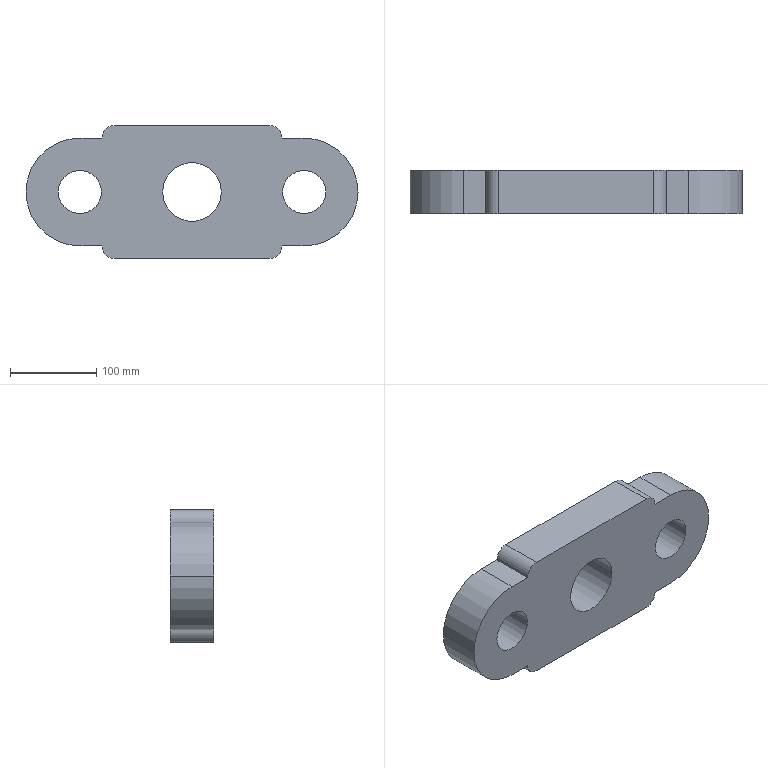Part | STEP file | Input 1-2 | 1 solid | 22 faces | box 385 x 50.4 x 154 mm | volume 2171922 mm3 | cylinder 14 | plane 8 | commonest cylinder face diameters 29 x4 50 x4 125 x4 68 x2
STEP:
#1=CARTESIAN_POINT('',(-556.359,1804.418,3172.342));
#2=VERTEX_POINT('',#1);
#3=CARTESIAN_POINT('',(-618.859,1804.418,3109.842));
#4=VERTEX_POINT('',#3);
#5=CARTESIAN_POINT('',(-618.859,1804.418,3172.342));
#6=DIRECTION('',(0.,1.,0.));
#7=DIRECTION('',(-1.,0.,0.));
#8=AXIS2_PLACEMENT_3D('',#5,#6,#7);
#9=CIRCLE('',#8,62.5);
#10=EDGE_CURVE('',#2,#4,#9,.T.);
#11=ORIENTED_EDGE('',*,*,#10,.F.);
#12=CARTESIAN_POINT('',(-556.359,1754.018,3172.342));
#13=VERTEX_POINT('',#12);
#14=CARTESIAN_POINT('',(-556.359,1804.418,3172.342));
#15=DIRECTION('',(0.,-1.,0.));
#16=VECTOR('',#15,1000.);
#17=LINE('',#14,#16);
#18=EDGE_CURVE('',#2,#13,#17,.T.);
#19=ORIENTED_EDGE('',*,*,#18,.T.);
#20=CARTESIAN_POINT('',(-618.859,1754.018,3109.842));
#21=VERTEX_POINT('',#20);
#22=CARTESIAN_POINT('',(-618.859,1754.018,3172.342));
#23=DIRECTION('',(0.,1.,0.));
#24=DIRECTION('',(-1.,0.,0.));
#25=AXIS2_PLACEMENT_3D('',#22,#23,#24);
#26=CIRCLE('',#25,62.5);
#27=EDGE_CURVE('',#13,#21,#26,.T.);
#28=ORIENTED_EDGE('',*,*,#27,.T.);
#29=CARTESIAN_POINT('',(-618.859,1804.418,3109.842));
#30=DIRECTION('',(0.,-1.,0.));
#31=VECTOR('',#30,1000.);
#32=LINE('',#29,#31);
#33=EDGE_CURVE('',#4,#21,#32,.T.);
#34=ORIENTED_EDGE('',*,*,#33,.F.);
#35=EDGE_LOOP('',(#11,#19,#28,#34));
#36=FACE_OUTER_BOUND('',#35,.T.);
#37=CARTESIAN_POINT('',(-618.859,1804.418,3172.342));
#38=DIRECTION('',(0.,-1.,0.));
#39=DIRECTION('',(1.,0.,0.));
#40=AXIS2_PLACEMENT_3D('',#37,#38,#39);
#41=CYLINDRICAL_SURFACE('',#40,62.5);
#42=ADVANCED_FACE('',(#36),#41,.T.);
#43=CARTESIAN_POINT('',(-782.859,1804.418,3172.342));
#44=VERTEX_POINT('',#43);
#45=CARTESIAN_POINT('',(-714.859,1804.418,3172.342));
#46=VERTEX_POINT('',#45);
#47=CARTESIAN_POINT('',(-748.859,1804.418,3172.342));
#48=DIRECTION('',(0.,1.,0.));
#49=DIRECTION('',(1.,0.,0.));
#50=AXIS2_PLACEMENT_3D('',#47,#48,#49);
#51=CIRCLE('',#50,34.);
#52=EDGE_CURVE('',#44,#46,#51,.T.);
#53=ORIENTED_EDGE('',*,*,#52,.T.);
#54=CARTESIAN_POINT('',(-714.859,1754.018,3172.342));
#55=VERTEX_POINT('',#54);
#56=CARTESIAN_POINT('',(-714.859,1804.418,3172.342));
#57=DIRECTION('',(0.,1.,0.));
#58=VECTOR('',#57,1000.);
#59=LINE('',#56,#58);
#60=EDGE_CURVE('',#55,#46,#59,.T.);
#61=ORIENTED_EDGE('',*,*,#60,.F.);
#62=CARTESIAN_POINT('',(-782.859,1754.018,3172.342));
#63=VERTEX_POINT('',#62);
#64=CARTESIAN_POINT('',(-748.859,1754.018,3172.342));
#65=DIRECTION('',(0.,1.,0.));
#66=DIRECTION('',(1.,0.,0.));
#67=AXIS2_PLACEMENT_3D('',#64,#65,#66);
#68=CIRCLE('',#67,34.);
#69=EDGE_CURVE('',#63,#55,#68,.T.);
#70=ORIENTED_EDGE('',*,*,#69,.F.);
#71=CARTESIAN_POINT('',(-782.859,1804.418,3172.342));
#72=DIRECTION('',(0.,1.,0.));
#73=VECTOR('',#72,1000.);
#74=LINE('',#71,#73);
#75=EDGE_CURVE('',#63,#44,#74,.T.);
#76=ORIENTED_EDGE('',*,*,#75,.T.);
#77=EDGE_LOOP('',(#53,#61,#70,#76));
#78=FACE_OUTER_BOUND('',#77,.T.);
#79=CARTESIAN_POINT('',(-748.859,1804.418,3172.342));
#80=DIRECTION('',(0.,-1.,0.));
#81=DIRECTION('',(1.,0.,0.));
#82=AXIS2_PLACEMENT_3D('',#79,#80,#81);
#83=CYLINDRICAL_SURFACE('',#82,34.);
#84=ADVANCED_FACE('',(#78),#83,.F.);
#85=CARTESIAN_POINT('',(-643.859,1804.418,3172.342));
#86=VERTEX_POINT('',#85);
#87=CARTESIAN_POINT('',(-593.859,1804.418,3172.342));
#88=VERTEX_POINT('',#87);
#89=CARTESIAN_POINT('',(-618.859,1804.418,3172.342));
#90=DIRECTION('',(0.,1.,0.));
#91=DIRECTION('',(1.,0.,0.));
#92=AXIS2_PLACEMENT_3D('',#89,#90,#91);
#93=CIRCLE('',#92,25.);
#94=EDGE_CURVE('',#86,#88,#93,.T.);
#95=ORIENTED_EDGE('',*,*,#94,.T.);
#96=CARTESIAN_POINT('',(-593.859,1754.018,3172.342));
#97=VERTEX_POINT('',#96);
#98=CARTESIAN_POINT('',(-593.859,1804.418,3172.342));
#99=DIRECTION('',(0.,1.,0.));
#100=VECTOR('',#99,1000.);
#101=LINE('',#98,#100);
#102=EDGE_CURVE('',#97,#88,#101,.T.);
#103=ORIENTED_EDGE('',*,*,#102,.F.);
#104=CARTESIAN_POINT('',(-643.859,1754.018,3172.342));
#105=VERTEX_POINT('',#104);
#106=CARTESIAN_POINT('',(-618.859,1754.018,3172.342));
#107=DIRECTION('',(0.,1.,0.));
#108=DIRECTION('',(1.,0.,0.));
#109=AXIS2_PLACEMENT_3D('',#106,#107,#108);
#110=CIRCLE('',#109,25.);
#111=EDGE_CURVE('',#105,#97,#110,.T.);
#112=ORIENTED_EDGE('',*,*,#111,.F.);
#113=CARTESIAN_POINT('',(-643.859,1804.418,3172.342));
#114=DIRECTION('',(0.,1.,0.));
#115=VECTOR('',#114,1000.);
#116=LINE('',#113,#115);
#117=EDGE_CURVE('',#105,#86,#116,.T.);
#118=ORIENTED_EDGE('',*,*,#117,.T.);
#119=EDGE_LOOP('',(#95,#103,#112,#118));
#120=FACE_OUTER_BOUND('',#119,.T.);
#121=CARTESIAN_POINT('',(-618.859,1804.418,3172.342));
#122=DIRECTION('',(0.,-1.,0.));
#123=DIRECTION('',(1.,0.,0.));
#124=AXIS2_PLACEMENT_3D('',#121,#122,#123);
#125=CYLINDRICAL_SURFACE('',#124,25.);
#126=ADVANCED_FACE('',(#120),#125,.F.);
#127=CARTESIAN_POINT('',(-903.859,1804.418,3172.342));
#128=VERTEX_POINT('',#127);
#129=CARTESIAN_POINT('',(-853.859,1804.418,3172.342));
#130=VERTEX_POINT('',#129);
#131=CARTESIAN_POINT('',(-878.859,1804.418,3172.342));
#132=DIRECTION('',(0.,1.,0.));
#133=DIRECTION('',(1.,0.,0.));
#134=AXIS2_PLACEMENT_3D('',#131,#132,#133);
#135=CIRCLE('',#134,25.);
#136=EDGE_CURVE('',#128,#130,#135,.T.);
#137=ORIENTED_EDGE('',*,*,#136,.T.);
#138=CARTESIAN_POINT('',(-853.859,1754.018,3172.342));
#139=VERTEX_POINT('',#138);
#140=CARTESIAN_POINT('',(-853.859,1804.418,3172.342));
#141=DIRECTION('',(0.,1.,0.));
#142=VECTOR('',#141,1000.);
#143=LINE('',#140,#142);
#144=EDGE_CURVE('',#139,#130,#143,.T.);
#145=ORIENTED_EDGE('',*,*,#144,.F.);
#146=CARTESIAN_POINT('',(-903.859,1754.018,3172.342));
#147=VERTEX_POINT('',#146);
#148=CARTESIAN_POINT('',(-878.859,1754.018,3172.342));
#149=DIRECTION('',(0.,1.,0.));
#150=DIRECTION('',(1.,0.,0.));
#151=AXIS2_PLACEMENT_3D('',#148,#149,#150);
#152=CIRCLE('',#151,25.);
#153=EDGE_CURVE('',#147,#139,#152,.T.);
#154=ORIENTED_EDGE('',*,*,#153,.F.);
#155=CARTESIAN_POINT('',(-903.859,1804.418,3172.342));
#156=DIRECTION('',(0.,1.,0.));
#157=VECTOR('',#156,1000.);
#158=LINE('',#155,#157);
#159=EDGE_CURVE('',#147,#128,#158,.T.);
#160=ORIENTED_EDGE('',*,*,#159,.T.);
#161=EDGE_LOOP('',(#137,#145,#154,#160));
#162=FACE_OUTER_BOUND('',#161,.T.);
#163=CARTESIAN_POINT('',(-878.859,1804.418,3172.342));
#164=DIRECTION('',(0.,-1.,0.));
#165=DIRECTION('',(1.,0.,0.));
#166=AXIS2_PLACEMENT_3D('',#163,#164,#165);
#167=CYLINDRICAL_SURFACE('',#166,25.);
#168=ADVANCED_FACE('',(#162),#167,.F.);
#169=CARTESIAN_POINT('',(-941.359,1804.418,3172.342));
#170=VERTEX_POINT('',#169);
#171=CARTESIAN_POINT('',(-878.859,1804.418,3234.842));
#172=VERTEX_POINT('',#171);
#173=CARTESIAN_POINT('',(-878.859,1804.418,3172.342));
#174=DIRECTION('',(0.,1.,0.));
#175=DIRECTION('',(1.,0.,0.));
#176=AXIS2_PLACEMENT_3D('',#173,#174,#175);
#177=CIRCLE('',#176,62.5);
#178=EDGE_CURVE('',#170,#172,#177,.T.);
#179=ORIENTED_EDGE('',*,*,#178,.F.);
#180=CARTESIAN_POINT('',(-941.359,1754.018,3172.342));
#181=VERTEX_POINT('',#180);
#182=CARTESIAN_POINT('',(-941.359,1804.418,3172.342));
#183=DIRECTION('',(0.,-1.,0.));
#184=VECTOR('',#183,1000.);
#185=LINE('',#182,#184);
#186=EDGE_CURVE('',#170,#181,#185,.T.);
#187=ORIENTED_EDGE('',*,*,#186,.T.);
#188=CARTESIAN_POINT('',(-878.859,1754.018,3234.842));
#189=VERTEX_POINT('',#188);
#190=CARTESIAN_POINT('',(-878.859,1754.018,3172.342));
#191=DIRECTION('',(0.,1.,0.));
#192=DIRECTION('',(1.,0.,0.));
#193=AXIS2_PLACEMENT_3D('',#190,#191,#192);
#194=CIRCLE('',#193,62.5);
#195=EDGE_CURVE('',#181,#189,#194,.T.);
#196=ORIENTED_EDGE('',*,*,#195,.T.);
#197=CARTESIAN_POINT('',(-878.859,1804.418,3234.842));
#198=DIRECTION('',(0.,-1.,0.));
#199=VECTOR('',#198,1000.);
#200=LINE('',#197,#199);
#201=EDGE_CURVE('',#172,#189,#200,.T.);
#202=ORIENTED_EDGE('',*,*,#201,.F.);
#203=EDGE_LOOP('',(#179,#187,#196,#202));
#204=FACE_OUTER_BOUND('',#203,.T.);
#205=CARTESIAN_POINT('',(-878.859,1804.418,3172.342));
#206=DIRECTION('',(0.,-1.,0.));
#207=DIRECTION('',(1.,0.,0.));
#208=AXIS2_PLACEMENT_3D('',#205,#206,#207);
#209=CYLINDRICAL_SURFACE('',#208,62.5);
#210=ADVANCED_FACE('',(#204),#209,.T.);
#211=ORIENTED_EDGE('',*,*,#94,.F.);
#212=CARTESIAN_POINT('',(-618.859,1804.418,3172.342));
#213=DIRECTION('',(0.,1.,0.));
#214=DIRECTION('',(1.,0.,0.));
#215=AXIS2_PLACEMENT_3D('',#212,#213,#214);
#216=CIRCLE('',#215,25.);
#217=EDGE_CURVE('',#88,#86,#216,.T.);
#218=ORIENTED_EDGE('',*,*,#217,.F.);
#219=EDGE_LOOP('',(#211,#218));
#220=FACE_BOUND('',#219,.T.);
#221=CARTESIAN_POINT('',(-878.859,1804.418,3109.842));
#222=VERTEX_POINT('',#221);
#223=CARTESIAN_POINT('',(-878.859,1804.418,3172.342));
#224=DIRECTION('',(0.,1.,0.));
#225=DIRECTION('',(1.,0.,0.));
#226=AXIS2_PLACEMENT_3D('',#223,#224,#225);
#227=CIRCLE('',#226,62.5);
#228=EDGE_CURVE('',#222,#170,#227,.T.);
#229=ORIENTED_EDGE('',*,*,#228,.T.);
#230=ORIENTED_EDGE('',*,*,#178,.T.);
#231=CARTESIAN_POINT('',(-853.359,1804.418,3234.842));
#232=VERTEX_POINT('',#231);
#233=CARTESIAN_POINT('',(-878.859,1804.418,3234.842));
#234=DIRECTION('',(1.,0.,0.));
#235=VECTOR('',#234,1000.);
#236=LINE('',#233,#235);
#237=EDGE_CURVE('',#172,#232,#236,.T.);
#238=ORIENTED_EDGE('',*,*,#237,.T.);
#239=CARTESIAN_POINT('',(-838.859,1804.418,3249.342));
#240=VERTEX_POINT('',#239);
#241=CARTESIAN_POINT('',(-838.859,1804.418,3234.842));
#242=DIRECTION('',(0.,1.,0.));
#243=DIRECTION('',(-1.,0.,0.));
#244=AXIS2_PLACEMENT_3D('',#241,#242,#243);
#245=CIRCLE('',#244,14.5);
#246=EDGE_CURVE('',#232,#240,#245,.T.);
#247=ORIENTED_EDGE('',*,*,#246,.T.);
#248=CARTESIAN_POINT('',(-658.859,1804.418,3249.342));
#249=VERTEX_POINT('',#248);
#250=CARTESIAN_POINT('',(-658.859,1804.418,3249.342));
#251=DIRECTION('',(1.,0.,0.));
#252=VECTOR('',#251,1000.);
#253=LINE('',#250,#252);
#254=EDGE_CURVE('',#240,#249,#253,.T.);
#255=ORIENTED_EDGE('',*,*,#254,.T.);
#256=CARTESIAN_POINT('',(-644.359,1804.418,3234.842));
#257=VERTEX_POINT('',#256);
#258=CARTESIAN_POINT('',(-658.859,1804.418,3234.842));
#259=DIRECTION('',(0.,1.,0.));
#260=DIRECTION('',(1.,0.,0.));
#261=AXIS2_PLACEMENT_3D('',#258,#259,#260);
#262=CIRCLE('',#261,14.5);
#263=EDGE_CURVE('',#249,#257,#262,.T.);
#264=ORIENTED_EDGE('',*,*,#263,.T.);
#265=CARTESIAN_POINT('',(-618.859,1804.418,3234.842));
#266=VERTEX_POINT('',#265);
#267=CARTESIAN_POINT('',(-618.859,1804.418,3234.842));
#268=DIRECTION('',(1.,0.,0.));
#269=VECTOR('',#268,1000.);
#270=LINE('',#267,#269);
#271=EDGE_CURVE('',#257,#266,#270,.T.);
#272=ORIENTED_EDGE('',*,*,#271,.T.);
#273=CARTESIAN_POINT('',(-618.859,1804.418,3172.342));
#274=DIRECTION('',(0.,1.,0.));
#275=DIRECTION('',(-1.,0.,0.));
#276=AXIS2_PLACEMENT_3D('',#273,#274,#275);
#277=CIRCLE('',#276,62.5);
#278=EDGE_CURVE('',#266,#2,#277,.T.);
#279=ORIENTED_EDGE('',*,*,#278,.T.);
#280=ORIENTED_EDGE('',*,*,#10,.T.);
#281=CARTESIAN_POINT('',(-644.359,1804.418,3109.842));
#282=VERTEX_POINT('',#281);
#283=CARTESIAN_POINT('',(-618.859,1804.418,3109.842));
#284=DIRECTION('',(-1.,0.,0.));
#285=VECTOR('',#284,1000.);
#286=LINE('',#283,#285);
#287=EDGE_CURVE('',#4,#282,#286,.T.);
#288=ORIENTED_EDGE('',*,*,#287,.T.);
#289=CARTESIAN_POINT('',(-658.859,1804.418,3095.342));
#290=VERTEX_POINT('',#289);
#291=CARTESIAN_POINT('',(-658.859,1804.418,3109.842));
#292=DIRECTION('',(0.,1.,0.));
#293=DIRECTION('',(-1.,0.,0.));
#294=AXIS2_PLACEMENT_3D('',#291,#292,#293);
#295=CIRCLE('',#294,14.5);
#296=EDGE_CURVE('',#282,#290,#295,.T.);
#297=ORIENTED_EDGE('',*,*,#296,.T.);
#298=CARTESIAN_POINT('',(-838.859,1804.418,3095.342));
#299=VERTEX_POINT('',#298);
#300=CARTESIAN_POINT('',(-658.859,1804.418,3095.342));
#301=DIRECTION('',(-1.,0.,0.));
#302=VECTOR('',#301,1000.);
#303=LINE('',#300,#302);
#304=EDGE_CURVE('',#290,#299,#303,.T.);
#305=ORIENTED_EDGE('',*,*,#304,.T.);
#306=CARTESIAN_POINT('',(-853.359,1804.418,3109.842));
#307=VERTEX_POINT('',#306);
#308=CARTESIAN_POINT('',(-838.859,1804.418,3109.842));
#309=DIRECTION('',(0.,1.,0.));
#310=DIRECTION('',(1.,0.,0.));
#311=AXIS2_PLACEMENT_3D('',#308,#309,#310);
#312=CIRCLE('',#311,14.5);
#313=EDGE_CURVE('',#299,#307,#312,.T.);
#314=ORIENTED_EDGE('',*,*,#313,.T.);
#315=CARTESIAN_POINT('',(-878.859,1804.418,3109.842));
#316=DIRECTION('',(-1.,0.,0.));
#317=VECTOR('',#316,1000.);
#318=LINE('',#315,#317);
#319=EDGE_CURVE('',#307,#222,#318,.T.);
#320=ORIENTED_EDGE('',*,*,#319,.T.);
#321=EDGE_LOOP('',(#229,#230,#238,#247,#255,#264,#272,#279,#280,#288,#297,#305,#314,#320));
#322=FACE_OUTER_BOUND('',#321,.T.);
#323=ORIENTED_EDGE('',*,*,#136,.F.);
#324=CARTESIAN_POINT('',(-878.859,1804.418,3172.342));
#325=DIRECTION('',(0.,1.,0.));
#326=DIRECTION('',(1.,0.,0.));
#327=AXIS2_PLACEMENT_3D('',#324,#325,#326);
#328=CIRCLE('',#327,25.);
#329=EDGE_CURVE('',#130,#128,#328,.T.);
#330=ORIENTED_EDGE('',*,*,#329,.F.);
#331=EDGE_LOOP('',(#323,#330));
#332=FACE_BOUND('',#331,.T.);
#333=ORIENTED_EDGE('',*,*,#52,.F.);
#334=CARTESIAN_POINT('',(-748.859,1804.418,3172.342));
#335=DIRECTION('',(0.,1.,0.));
#336=DIRECTION('',(1.,0.,0.));
#337=AXIS2_PLACEMENT_3D('',#334,#335,#336);
#338=CIRCLE('',#337,34.);
#339=EDGE_CURVE('',#46,#44,#338,.T.);
#340=ORIENTED_EDGE('',*,*,#339,.F.);
#341=EDGE_LOOP('',(#333,#340));
#342=FACE_BOUND('',#341,.T.);
#343=CARTESIAN_POINT('',(-878.859,1804.418,3172.342));
#344=DIRECTION('',(0.,1.,0.));
#345=DIRECTION('',(-1.,0.,0.));
#346=AXIS2_PLACEMENT_3D('',#343,#344,#345);
#347=PLANE('',#346);
#348=ADVANCED_FACE('',(#220,#322,#332,#342),#347,.T.);
#349=ORIENTED_EDGE('',*,*,#111,.T.);
#350=CARTESIAN_POINT('',(-618.859,1754.018,3172.342));
#351=DIRECTION('',(0.,1.,0.));
#352=DIRECTION('',(1.,0.,0.));
#353=AXIS2_PLACEMENT_3D('',#350,#351,#352);
#354=CIRCLE('',#353,25.);
#355=EDGE_CURVE('',#97,#105,#354,.T.);
#356=ORIENTED_EDGE('',*,*,#355,.T.);
#357=EDGE_LOOP('',(#349,#356));
#358=FACE_BOUND('',#357,.T.);
#359=CARTESIAN_POINT('',(-878.859,1754.018,3109.842));
#360=VERTEX_POINT('',#359);
#361=CARTESIAN_POINT('',(-878.859,1754.018,3172.342));
#362=DIRECTION('',(0.,1.,0.));
#363=DIRECTION('',(1.,0.,0.));
#364=AXIS2_PLACEMENT_3D('',#361,#362,#363);
#365=CIRCLE('',#364,62.5);
#366=EDGE_CURVE('',#360,#181,#365,.T.);
#367=ORIENTED_EDGE('',*,*,#366,.F.);
#368=CARTESIAN_POINT('',(-853.359,1754.018,3109.842));
#369=VERTEX_POINT('',#368);
#370=CARTESIAN_POINT('',(-878.859,1754.018,3109.842));
#371=DIRECTION('',(-1.,0.,0.));
#372=VECTOR('',#371,1000.);
#373=LINE('',#370,#372);
#374=EDGE_CURVE('',#369,#360,#373,.T.);
#375=ORIENTED_EDGE('',*,*,#374,.F.);
#376=CARTESIAN_POINT('',(-838.859,1754.018,3095.342));
#377=VERTEX_POINT('',#376);
#378=CARTESIAN_POINT('',(-838.859,1754.018,3109.842));
#379=DIRECTION('',(0.,1.,0.));
#380=DIRECTION('',(1.,0.,0.));
#381=AXIS2_PLACEMENT_3D('',#378,#379,#380);
#382=CIRCLE('',#381,14.5);
#383=EDGE_CURVE('',#377,#369,#382,.T.);
#384=ORIENTED_EDGE('',*,*,#383,.F.);
#385=CARTESIAN_POINT('',(-658.859,1754.018,3095.342));
#386=VERTEX_POINT('',#385);
#387=CARTESIAN_POINT('',(-658.859,1754.018,3095.342));
#388=DIRECTION('',(-1.,0.,0.));
#389=VECTOR('',#388,1000.);
#390=LINE('',#387,#389);
#391=EDGE_CURVE('',#386,#377,#390,.T.);
#392=ORIENTED_EDGE('',*,*,#391,.F.);
#393=CARTESIAN_POINT('',(-644.359,1754.018,3109.842));
#394=VERTEX_POINT('',#393);
#395=CARTESIAN_POINT('',(-658.859,1754.018,3109.842));
#396=DIRECTION('',(0.,1.,0.));
#397=DIRECTION('',(-1.,0.,0.));
#398=AXIS2_PLACEMENT_3D('',#395,#396,#397);
#399=CIRCLE('',#398,14.5);
#400=EDGE_CURVE('',#394,#386,#399,.T.);
#401=ORIENTED_EDGE('',*,*,#400,.F.);
#402=CARTESIAN_POINT('',(-618.859,1754.018,3109.842));
#403=DIRECTION('',(-1.,0.,0.));
#404=VECTOR('',#403,1000.);
#405=LINE('',#402,#404);
#406=EDGE_CURVE('',#21,#394,#405,.T.);
#407=ORIENTED_EDGE('',*,*,#406,.F.);
#408=ORIENTED_EDGE('',*,*,#27,.F.);
#409=CARTESIAN_POINT('',(-618.859,1754.018,3234.842));
#410=VERTEX_POINT('',#409);
#411=CARTESIAN_POINT('',(-618.859,1754.018,3172.342));
#412=DIRECTION('',(0.,1.,0.));
#413=DIRECTION('',(-1.,0.,0.));
#414=AXIS2_PLACEMENT_3D('',#411,#412,#413);
#415=CIRCLE('',#414,62.5);
#416=EDGE_CURVE('',#410,#13,#415,.T.);
#417=ORIENTED_EDGE('',*,*,#416,.F.);
#418=CARTESIAN_POINT('',(-644.359,1754.018,3234.842));
#419=VERTEX_POINT('',#418);
#420=CARTESIAN_POINT('',(-618.859,1754.018,3234.842));
#421=DIRECTION('',(1.,0.,0.));
#422=VECTOR('',#421,1000.);
#423=LINE('',#420,#422);
#424=EDGE_CURVE('',#419,#410,#423,.T.);
#425=ORIENTED_EDGE('',*,*,#424,.F.);
#426=CARTESIAN_POINT('',(-658.859,1754.018,3249.342));
#427=VERTEX_POINT('',#426);
#428=CARTESIAN_POINT('',(-658.859,1754.018,3234.842));
#429=DIRECTION('',(0.,1.,0.));
#430=DIRECTION('',(1.,0.,0.));
#431=AXIS2_PLACEMENT_3D('',#428,#429,#430);
#432=CIRCLE('',#431,14.5);
#433=EDGE_CURVE('',#427,#419,#432,.T.);
#434=ORIENTED_EDGE('',*,*,#433,.F.);
#435=CARTESIAN_POINT('',(-838.859,1754.018,3249.342));
#436=VERTEX_POINT('',#435);
#437=CARTESIAN_POINT('',(-658.859,1754.018,3249.342));
#438=DIRECTION('',(1.,0.,0.));
#439=VECTOR('',#438,1000.);
#440=LINE('',#437,#439);
#441=EDGE_CURVE('',#436,#427,#440,.T.);
#442=ORIENTED_EDGE('',*,*,#441,.F.);
#443=CARTESIAN_POINT('',(-853.359,1754.018,3234.842));
#444=VERTEX_POINT('',#443);
#445=CARTESIAN_POINT('',(-838.859,1754.018,3234.842));
#446=DIRECTION('',(0.,1.,0.));
#447=DIRECTION('',(-1.,0.,0.));
#448=AXIS2_PLACEMENT_3D('',#445,#446,#447);
#449=CIRCLE('',#448,14.5);
#450=EDGE_CURVE('',#444,#436,#449,.T.);
#451=ORIENTED_EDGE('',*,*,#450,.F.);
#452=CARTESIAN_POINT('',(-878.859,1754.018,3234.842));
#453=DIRECTION('',(1.,0.,0.));
#454=VECTOR('',#453,1000.);
#455=LINE('',#452,#454);
#456=EDGE_CURVE('',#189,#444,#455,.T.);
#457=ORIENTED_EDGE('',*,*,#456,.F.);
#458=ORIENTED_EDGE('',*,*,#195,.F.);
#459=EDGE_LOOP('',(#367,#375,#384,#392,#401,#407,#408,#417,#425,#434,#442,#451,#457,#458));
#460=FACE_OUTER_BOUND('',#459,.T.);
#461=ORIENTED_EDGE('',*,*,#153,.T.);
#462=CARTESIAN_POINT('',(-878.859,1754.018,3172.342));
#463=DIRECTION('',(0.,1.,0.));
#464=DIRECTION('',(1.,0.,0.));
#465=AXIS2_PLACEMENT_3D('',#462,#463,#464);
#466=CIRCLE('',#465,25.);
#467=EDGE_CURVE('',#139,#147,#466,.T.);
#468=ORIENTED_EDGE('',*,*,#467,.T.);
#469=EDGE_LOOP('',(#461,#468));
#470=FACE_BOUND('',#469,.T.);
#471=ORIENTED_EDGE('',*,*,#69,.T.);
#472=CARTESIAN_POINT('',(-748.859,1754.018,3172.342));
#473=DIRECTION('',(0.,1.,0.));
#474=DIRECTION('',(1.,0.,0.));
#475=AXIS2_PLACEMENT_3D('',#472,#473,#474);
#476=CIRCLE('',#475,34.);
#477=EDGE_CURVE('',#55,#63,#476,.T.);
#478=ORIENTED_EDGE('',*,*,#477,.T.);
#479=EDGE_LOOP('',(#471,#478));
#480=FACE_BOUND('',#479,.T.);
#481=CARTESIAN_POINT('',(-878.859,1754.018,3172.342));
#482=DIRECTION('',(0.,1.,0.));
#483=DIRECTION('',(-1.,0.,0.));
#484=AXIS2_PLACEMENT_3D('',#481,#482,#483);
#485=PLANE('',#484);
#486=ADVANCED_FACE('',(#358,#460,#470,#480),#485,.F.);
#487=ORIENTED_EDGE('',*,*,#186,.F.);
#488=ORIENTED_EDGE('',*,*,#228,.F.);
#489=CARTESIAN_POINT('',(-878.859,1804.418,3109.842));
#490=DIRECTION('',(0.,-1.,0.));
#491=VECTOR('',#490,1000.);
#492=LINE('',#489,#491);
#493=EDGE_CURVE('',#222,#360,#492,.T.);
#494=ORIENTED_EDGE('',*,*,#493,.T.);
#495=ORIENTED_EDGE('',*,*,#366,.T.);
#496=EDGE_LOOP('',(#487,#488,#494,#495));
#497=FACE_OUTER_BOUND('',#496,.T.);
#498=CARTESIAN_POINT('',(-878.859,1804.418,3172.342));
#499=DIRECTION('',(0.,-1.,0.));
#500=DIRECTION('',(1.,0.,0.));
#501=AXIS2_PLACEMENT_3D('',#498,#499,#500);
#502=CYLINDRICAL_SURFACE('',#501,62.5);
#503=ADVANCED_FACE('',(#497),#502,.T.);
#504=ORIENTED_EDGE('',*,*,#456,.T.);
#505=CARTESIAN_POINT('',(-853.359,1804.418,3234.842));
#506=DIRECTION('',(0.,-1.,0.));
#507=VECTOR('',#506,1000.);
#508=LINE('',#505,#507);
#509=EDGE_CURVE('',#232,#444,#508,.T.);
#510=ORIENTED_EDGE('',*,*,#509,.F.);
#511=ORIENTED_EDGE('',*,*,#237,.F.);
#512=ORIENTED_EDGE('',*,*,#201,.T.);
#513=EDGE_LOOP('',(#504,#510,#511,#512));
#514=FACE_OUTER_BOUND('',#513,.T.);
#515=CARTESIAN_POINT('',(-878.859,1804.418,3234.842));
#516=DIRECTION('',(0.,0.,-1.));
#517=DIRECTION('',(0.,-1.,0.));
#518=AXIS2_PLACEMENT_3D('',#515,#516,#517);
#519=PLANE('',#518);
#520=ADVANCED_FACE('',(#514),#519,.F.);
#521=ORIENTED_EDGE('',*,*,#450,.T.);
#522=CARTESIAN_POINT('',(-838.859,1804.418,3249.342));
#523=DIRECTION('',(0.,-1.,0.));
#524=VECTOR('',#523,1000.);
#525=LINE('',#522,#524);
#526=EDGE_CURVE('',#240,#436,#525,.T.);
#527=ORIENTED_EDGE('',*,*,#526,.F.);
#528=ORIENTED_EDGE('',*,*,#246,.F.);
#529=ORIENTED_EDGE('',*,*,#509,.T.);
#530=EDGE_LOOP('',(#521,#527,#528,#529));
#531=FACE_OUTER_BOUND('',#530,.T.);
#532=CARTESIAN_POINT('',(-838.859,1804.418,3234.842));
#533=DIRECTION('',(0.,-1.,0.));
#534=DIRECTION('',(1.,0.,0.));
#535=AXIS2_PLACEMENT_3D('',#532,#533,#534);
#536=CYLINDRICAL_SURFACE('',#535,14.5);
#537=ADVANCED_FACE('',(#531),#536,.T.);
#538=ORIENTED_EDGE('',*,*,#441,.T.);
#539=CARTESIAN_POINT('',(-658.859,1804.418,3249.342));
#540=DIRECTION('',(0.,-1.,0.));
#541=VECTOR('',#540,1000.);
#542=LINE('',#539,#541);
#543=EDGE_CURVE('',#249,#427,#542,.T.);
#544=ORIENTED_EDGE('',*,*,#543,.F.);
#545=ORIENTED_EDGE('',*,*,#254,.F.);
#546=ORIENTED_EDGE('',*,*,#526,.T.);
#547=EDGE_LOOP('',(#538,#544,#545,#546));
#548=FACE_OUTER_BOUND('',#547,.T.);
#549=CARTESIAN_POINT('',(-658.859,1804.418,3249.342));
#550=DIRECTION('',(0.,0.,-1.));
#551=DIRECTION('',(0.,-1.,0.));
#552=AXIS2_PLACEMENT_3D('',#549,#550,#551);
#553=PLANE('',#552);
#554=ADVANCED_FACE('',(#548),#553,.F.);
#555=ORIENTED_EDGE('',*,*,#433,.T.);
#556=CARTESIAN_POINT('',(-644.359,1804.418,3234.842));
#557=DIRECTION('',(0.,-1.,0.));
#558=VECTOR('',#557,1000.);
#559=LINE('',#556,#558);
#560=EDGE_CURVE('',#257,#419,#559,.T.);
#561=ORIENTED_EDGE('',*,*,#560,.F.);
#562=ORIENTED_EDGE('',*,*,#263,.F.);
#563=ORIENTED_EDGE('',*,*,#543,.T.);
#564=EDGE_LOOP('',(#555,#561,#562,#563));
#565=FACE_OUTER_BOUND('',#564,.T.);
#566=CARTESIAN_POINT('',(-658.859,1804.418,3234.842));
#567=DIRECTION('',(0.,-1.,0.));
#568=DIRECTION('',(1.,0.,0.));
#569=AXIS2_PLACEMENT_3D('',#566,#567,#568);
#570=CYLINDRICAL_SURFACE('',#569,14.5);
#571=ADVANCED_FACE('',(#565),#570,.T.);
#572=ORIENTED_EDGE('',*,*,#424,.T.);
#573=CARTESIAN_POINT('',(-618.859,1804.418,3234.842));
#574=DIRECTION('',(0.,-1.,0.));
#575=VECTOR('',#574,1000.);
#576=LINE('',#573,#575);
#577=EDGE_CURVE('',#266,#410,#576,.T.);
#578=ORIENTED_EDGE('',*,*,#577,.F.);
#579=ORIENTED_EDGE('',*,*,#271,.F.);
#580=ORIENTED_EDGE('',*,*,#560,.T.);
#581=EDGE_LOOP('',(#572,#578,#579,#580));
#582=FACE_OUTER_BOUND('',#581,.T.);
#583=CARTESIAN_POINT('',(-618.859,1804.418,3234.842));
#584=DIRECTION('',(0.,0.,-1.));
#585=DIRECTION('',(0.,-1.,0.));
#586=AXIS2_PLACEMENT_3D('',#583,#584,#585);
#587=PLANE('',#586);
#588=ADVANCED_FACE('',(#582),#587,.F.);
#589=ORIENTED_EDGE('',*,*,#18,.F.);
#590=ORIENTED_EDGE('',*,*,#278,.F.);
#591=ORIENTED_EDGE('',*,*,#577,.T.);
#592=ORIENTED_EDGE('',*,*,#416,.T.);
#593=EDGE_LOOP('',(#589,#590,#591,#592));
#594=FACE_OUTER_BOUND('',#593,.T.);
#595=CARTESIAN_POINT('',(-618.859,1804.418,3172.342));
#596=DIRECTION('',(0.,-1.,0.));
#597=DIRECTION('',(1.,0.,0.));
#598=AXIS2_PLACEMENT_3D('',#595,#596,#597);
#599=CYLINDRICAL_SURFACE('',#598,62.5);
#600=ADVANCED_FACE('',(#594),#599,.T.);
#601=ORIENTED_EDGE('',*,*,#406,.T.);
#602=CARTESIAN_POINT('',(-644.359,1804.418,3109.842));
#603=DIRECTION('',(0.,-1.,0.));
#604=VECTOR('',#603,1000.);
#605=LINE('',#602,#604);
#606=EDGE_CURVE('',#282,#394,#605,.T.);
#607=ORIENTED_EDGE('',*,*,#606,.F.);
#608=ORIENTED_EDGE('',*,*,#287,.F.);
#609=ORIENTED_EDGE('',*,*,#33,.T.);
#610=EDGE_LOOP('',(#601,#607,#608,#609));
#611=FACE_OUTER_BOUND('',#610,.T.);
#612=CARTESIAN_POINT('',(-618.859,1804.418,3109.842));
#613=DIRECTION('',(0.,0.,1.));
#614=DIRECTION('',(0.,1.,0.));
#615=AXIS2_PLACEMENT_3D('',#612,#613,#614);
#616=PLANE('',#615);
#617=ADVANCED_FACE('',(#611),#616,.F.);
#618=ORIENTED_EDGE('',*,*,#400,.T.);
#619=CARTESIAN_POINT('',(-658.859,1804.418,3095.342));
#620=DIRECTION('',(0.,-1.,0.));
#621=VECTOR('',#620,1000.);
#622=LINE('',#619,#621);
#623=EDGE_CURVE('',#290,#386,#622,.T.);
#624=ORIENTED_EDGE('',*,*,#623,.F.);
#625=ORIENTED_EDGE('',*,*,#296,.F.);
#626=ORIENTED_EDGE('',*,*,#606,.T.);
#627=EDGE_LOOP('',(#618,#624,#625,#626));
#628=FACE_OUTER_BOUND('',#627,.T.);
#629=CARTESIAN_POINT('',(-658.859,1804.418,3109.842));
#630=DIRECTION('',(0.,-1.,0.));
#631=DIRECTION('',(1.,0.,0.));
#632=AXIS2_PLACEMENT_3D('',#629,#630,#631);
#633=CYLINDRICAL_SURFACE('',#632,14.5);
#634=ADVANCED_FACE('',(#628),#633,.T.);
#635=ORIENTED_EDGE('',*,*,#391,.T.);
#636=CARTESIAN_POINT('',(-838.859,1804.418,3095.342));
#637=DIRECTION('',(0.,-1.,0.));
#638=VECTOR('',#637,1000.);
#639=LINE('',#636,#638);
#640=EDGE_CURVE('',#299,#377,#639,.T.);
#641=ORIENTED_EDGE('',*,*,#640,.F.);
#642=ORIENTED_EDGE('',*,*,#304,.F.);
#643=ORIENTED_EDGE('',*,*,#623,.T.);
#644=EDGE_LOOP('',(#635,#641,#642,#643));
#645=FACE_OUTER_BOUND('',#644,.T.);
#646=CARTESIAN_POINT('',(-658.859,1804.418,3095.342));
#647=DIRECTION('',(0.,0.,1.));
#648=DIRECTION('',(0.,1.,0.));
#649=AXIS2_PLACEMENT_3D('',#646,#647,#648);
#650=PLANE('',#649);
#651=ADVANCED_FACE('',(#645),#650,.F.);
#652=ORIENTED_EDGE('',*,*,#383,.T.);
#653=CARTESIAN_POINT('',(-853.359,1804.418,3109.842));
#654=DIRECTION('',(0.,-1.,0.));
#655=VECTOR('',#654,1000.);
#656=LINE('',#653,#655);
#657=EDGE_CURVE('',#307,#369,#656,.T.);
#658=ORIENTED_EDGE('',*,*,#657,.F.);
#659=ORIENTED_EDGE('',*,*,#313,.F.);
#660=ORIENTED_EDGE('',*,*,#640,.T.);
#661=EDGE_LOOP('',(#652,#658,#659,#660));
#662=FACE_OUTER_BOUND('',#661,.T.);
#663=CARTESIAN_POINT('',(-838.859,1804.418,3109.842));
#664=DIRECTION('',(0.,-1.,0.));
#665=DIRECTION('',(1.,0.,0.));
#666=AXIS2_PLACEMENT_3D('',#663,#664,#665);
#667=CYLINDRICAL_SURFACE('',#666,14.5);
#668=ADVANCED_FACE('',(#662),#667,.T.);
#669=ORIENTED_EDGE('',*,*,#374,.T.);
#670=ORIENTED_EDGE('',*,*,#493,.F.);
#671=ORIENTED_EDGE('',*,*,#319,.F.);
#672=ORIENTED_EDGE('',*,*,#657,.T.);
#673=EDGE_LOOP('',(#669,#670,#671,#672));
#674=FACE_OUTER_BOUND('',#673,.T.);
#675=CARTESIAN_POINT('',(-878.859,1804.418,3109.842));
#676=DIRECTION('',(0.,0.,1.));
#677=DIRECTION('',(0.,1.,0.));
#678=AXIS2_PLACEMENT_3D('',#675,#676,#677);
#679=PLANE('',#678);
#680=ADVANCED_FACE('',(#674),#679,.F.);
#681=ORIENTED_EDGE('',*,*,#144,.T.);
#682=ORIENTED_EDGE('',*,*,#329,.T.);
#683=ORIENTED_EDGE('',*,*,#159,.F.);
#684=ORIENTED_EDGE('',*,*,#467,.F.);
#685=EDGE_LOOP('',(#681,#682,#683,#684));
#686=FACE_OUTER_BOUND('',#685,.T.);
#687=CARTESIAN_POINT('',(-878.859,1804.418,3172.342));
#688=DIRECTION('',(0.,-1.,0.));
#689=DIRECTION('',(1.,0.,0.));
#690=AXIS2_PLACEMENT_3D('',#687,#688,#689);
#691=CYLINDRICAL_SURFACE('',#690,25.);
#692=ADVANCED_FACE('',(#686),#691,.F.);
#693=ORIENTED_EDGE('',*,*,#102,.T.);
#694=ORIENTED_EDGE('',*,*,#217,.T.);
#695=ORIENTED_EDGE('',*,*,#117,.F.);
#696=ORIENTED_EDGE('',*,*,#355,.F.);
#697=EDGE_LOOP('',(#693,#694,#695,#696));
#698=FACE_OUTER_BOUND('',#697,.T.);
#699=CARTESIAN_POINT('',(-618.859,1804.418,3172.342));
#700=DIRECTION('',(0.,-1.,0.));
#701=DIRECTION('',(1.,0.,0.));
#702=AXIS2_PLACEMENT_3D('',#699,#700,#701);
#703=CYLINDRICAL_SURFACE('',#702,25.);
#704=ADVANCED_FACE('',(#698),#703,.F.);
#705=ORIENTED_EDGE('',*,*,#60,.T.);
#706=ORIENTED_EDGE('',*,*,#339,.T.);
#707=ORIENTED_EDGE('',*,*,#75,.F.);
#708=ORIENTED_EDGE('',*,*,#477,.F.);
#709=EDGE_LOOP('',(#705,#706,#707,#708));
#710=FACE_OUTER_BOUND('',#709,.T.);
#711=CARTESIAN_POINT('',(-748.859,1804.418,3172.342));
#712=DIRECTION('',(0.,-1.,0.));
#713=DIRECTION('',(1.,0.,0.));
#714=AXIS2_PLACEMENT_3D('',#711,#712,#713);
#715=CYLINDRICAL_SURFACE('',#714,34.);
#716=ADVANCED_FACE('',(#710),#715,.F.);
#717=CLOSED_SHELL('',(#42,#84,#126,#168,#210,#348,#486,#503,#520,#537,#554,#571,#588,#600,#617,#634,#651,#668,#680,#692,#704,#716));
#718=MANIFOLD_SOLID_BREP('',#717);
#719=CARTESIAN_POINT('',(0.,0.,0.));
#720=DIRECTION('',(0.,0.,1.));
#721=DIRECTION('',(1.,0.,0.));
#722=AXIS2_PLACEMENT_3D('',#719,#720,#721);
#723=(LENGTH_UNIT()NAMED_UNIT(*)SI_UNIT(.MILLI.,.METRE.));
#724=UNCERTAINTY_MEASURE_WITH_UNIT(LENGTH_MEASURE(0.00001),#723,'','');
#725=(NAMED_UNIT(*)PLANE_ANGLE_UNIT()SI_UNIT($,.RADIAN.));
#726=(NAMED_UNIT(*)SI_UNIT($,.STERADIAN.)SOLID_ANGLE_UNIT());
#727=(GEOMETRIC_REPRESENTATION_CONTEXT(3)GLOBAL_UNCERTAINTY_ASSIGNED_CONTEXT((#724))GLOBAL_UNIT_ASSIGNED_CONTEXT((#723,#725,#726))REPRESENTATION_CONTEXT('',''));
#728=ADVANCED_BREP_SHAPE_REPRESENTATION('',(#718,#722),#727);